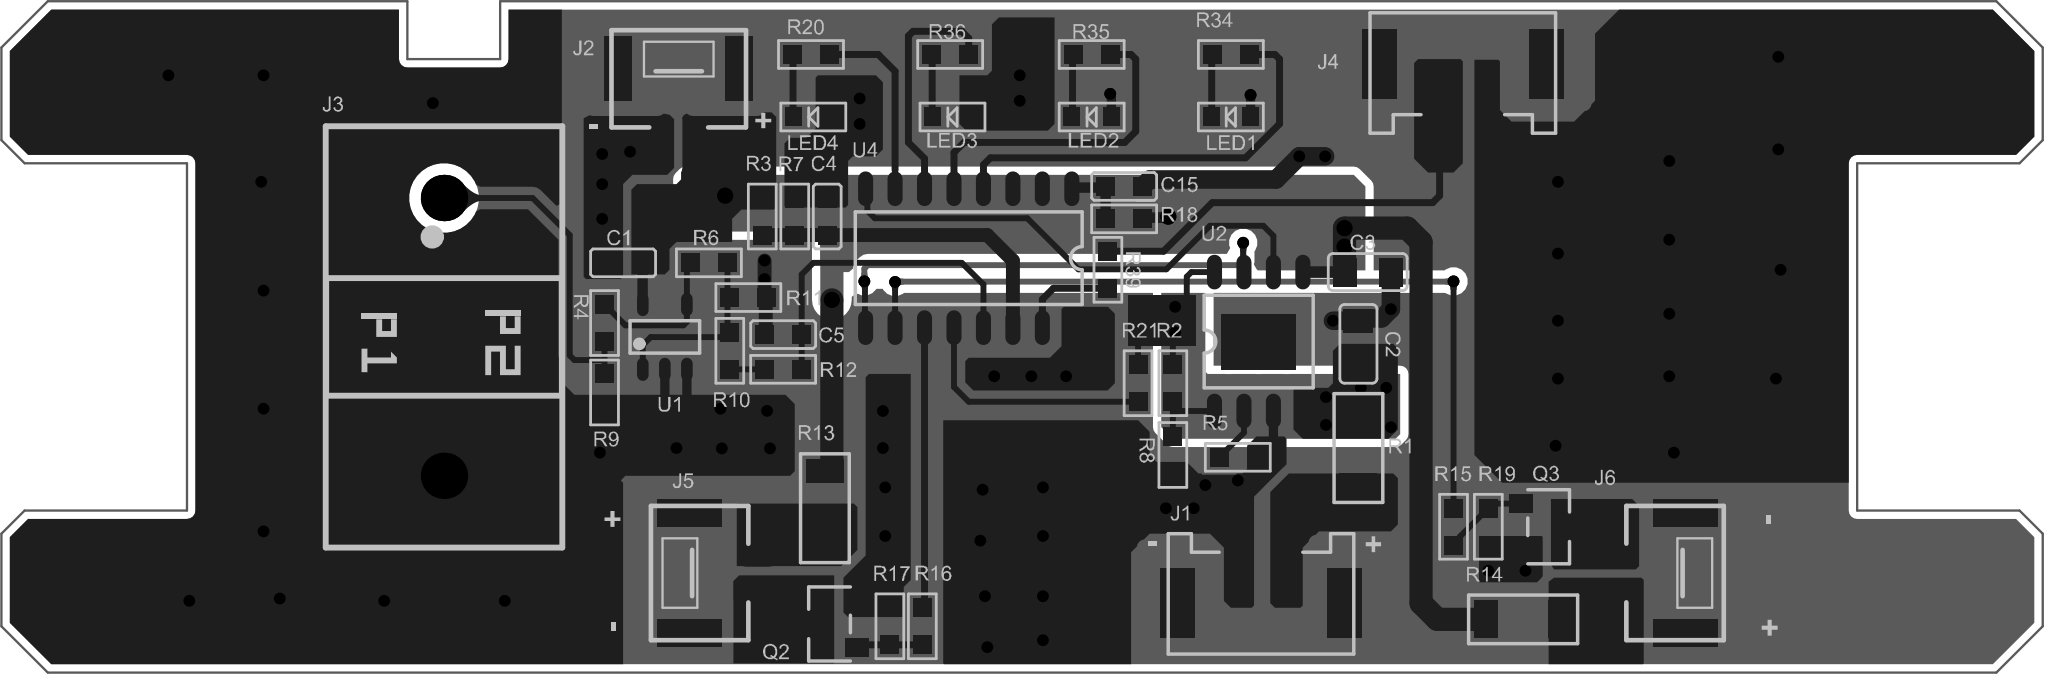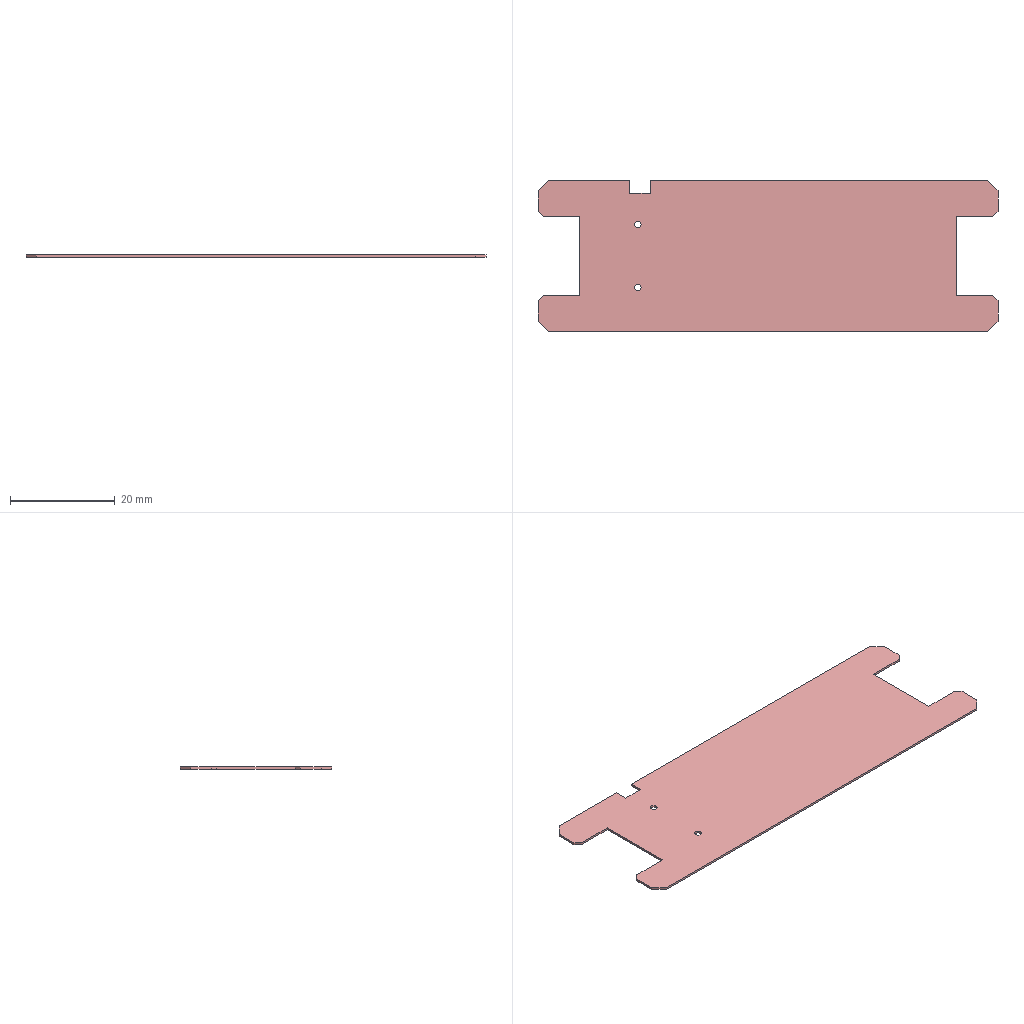Circuit board layout | Altium Designer | box 88 x 29 x 0.4 mm
Layer stack:
# Altium Designer layer stack of  (unit mm; dielectric type: 0 none, 1 core, 2 prepreg, 3 surface material)
index,name,kind,layer,copper_thickness_mm,dielectric_type,dielectric_thickness_mm,dielectric_material,dielectric_constant
0,Top Paste,other,,,,,,
1,Top Overlay,other,,,,,,
2,Top Solder,dielectric,,,3,0.0102,Solder Resist,3.5
3,Top Layer,copper,Top Layer,0.0356,,,,
4,Dielectric 1,dielectric,,,0,0.32,FR-4,4.8
5,Bottom Layer,copper,Bottom Layer,0.0356,,,,
6,Bottom Solder,dielectric,,,3,0.0102,Solder Resist,3.5
7,Bottom Overlay,other,,,,,,
8,Bottom Paste,other,,,,,,
# drill layer pairs: low layer,high layer
drill_pair,Top Layer,Bottom Layer
Part placement:
Designator,Comment,Layer,Footprint,Center-X(mm),Center-Y(mm),Rotation
C1,100nF/50V,TopLayer,C0603A,26.8,-9.3,0
U4,ZM072,TopLayer,SOP16L,41.7,-9.1,270
J3,Current sensor,TopLayer,IND-TH_L18.2-W10.2-P12.00-D0.9_ZHT103,19.08,-12.5,270
C15,1uF/10V,TopLayer,C0603A,48.4,-6,0
C3,10uF/10V,TopLayer,C0805A,58.9,-9.7,180
C2,10uF/10V,TopLayer,C0805A,58.5,-12.8,270
Q3,2N7002,TopLayer,SOT23-3L,66.7,-20.7,270
Q2,2N7002,TopLayer,SOT23-3L,35.7,-24.9,90
J6,Yellow LED,TopLayer,GH1.25-2PIN立贴带扣耐温260℃,71.125,-22.7,90
J5,Blue LED,TopLayer,GH1.25-2PIN立贴带扣耐温260℃,31.125,-22.7,270
J4,Test port,TopLayer,HY2.0WT-2A/P_Á¢Ìù´ø¿ÛÄÍÎÂ260¡æ,63,-1.9,180
J2,Battery,TopLayer,GH1.25-2PIN立贴带扣耐温260℃,29.2,-2.375,180
J1,Charge,TopLayer,HY2.0WT-2A/P_Á¢Ìù´ø¿ÛÄÍÎÂ260¡æ,54.3,-22.8,0
LED4,100%,TopLayer,LED0603A,35,-3,0
LED3,75%,TopLayer,LED0603A,41,-3,0
LED2,50%,TopLayer,LED0603A,47,-3,0
LED1,25%,TopLayer,LED0603A,53,-3,0
U2,4056,TopLayer,ESOP-8L,54.2,-12.7,90
U1,LM321,TopLayer,SOT23-5A,28.6,-12.5,90
R14,10R/1206,TopLayer,R1206A,65.6,-24.7,0
R13,10R/1206,TopLayer,R1206A,35.5,-19.9,270
R12,0R/0603,TopLayer,R0603A,33.7,-13.9,0
R11,10K/0603,TopLayer,R0603A,32.2,-10.8,0
R10,1K/0603,TopLayer,R0603A,31.4,-13.1,270
R9,2K/0603,TopLayer,R0603A,26,-14.9,270
R8,NC,TopLayer,R0603A,50.5,-17.6,90
R7,200K/0603 1%,TopLayer,R0603A,34.2,-7.3,270
R6,150K/0603,TopLayer,R0603A,30.5,-9.3,0
R5,1.2K/0603,TopLayer,R0603A,53.3,-17.7,180
R4,1K/0603,TopLayer,R0603A,26,-11.9,270
R3,510K/0603 1%,TopLayer,R0603A,32.8,-7.3,90
R2,NC,TopLayer,R0603A,50.5,-14.5,90
R1,0.5R/1206,TopLayer,R1206A,58.5,-17.3,90
C5,NC,TopLayer,C0603A,33.7,-12.4,0
C4,100nF/50V,TopLayer,C0603A,35.6,-7.3,270
R39,1K,TopLayer,R0603A,47.7,-9.6,90
R36,100R/5%,TopLayer,R0603A,40.9,-0.3,0
R35,100R/5%,TopLayer,R0603A,47,-0.3,0
R34,100R/5%,TopLayer,R0603A,53,-0.3,0
R21,NC,TopLayer,R0603A,49,-14.5,90
R20,100R/5%,TopLayer,R0603A,34.9,-0.3,0
R19,100K,TopLayer,R0603A,64.1,-20.7,90
R18,1R,TopLayer,R0603A,48.4,-7.4,180
R17,100K,TopLayer,R0603A,38.3,-25,270
R16,1K,TopLayer,R0603A,39.7,-25,90
R15,1K,TopLayer,R0603A,62.6,-20.7,90
Pad and via stacks:
# Altium Designer via and pad stacks of  (unit mm). Each distinct definition once, with the count of objects using it.
# via: kind,start_layer,end_layer,hole_mm,diameter_mm,mode(0 simple;1 top-mid-bottom;2 full stack),diameter_per_layer,count,example_net
# pad: kind,layer,hole_mm,hole_type(0 round;1 square;2 slot),plating,top_size,top_shape(1 round;2 rect;3 octagon;9 rounded rect),mid_size,bottom_size,mode,footprint,size_per_layer,count,example
pad,Top Layer,0,0,plated,1x1,1,1x1,1x1,0,,,2,3
pad,Top Layer,0,0,plated,3x1.5,2,3x1.5,3x1.5,0,HY2.0WT-2A/P \u00C1\u00A2\u00CC\u00F9\u00B4\u00F8\u00BF\u00DB\u00C4\u00CD\u00CE\u00C2260\u00A1\u00E6,,4,J4.0
pad,Top Layer,0,0,plated,4.5x0.8,1,4.5x0.8,4.5x0.8,0,HY2.0WT-2A/P \u00C1\u00A2\u00CC\u00F9\u00B4\u00F8\u00BF\u00DB\u00C4\u00CD\u00CE\u00C2260\u00A1\u00E6,,4,J4.1
pad,Top Layer,0,0,plated,0.7x0.8,2,0.7x0.8,0.7x0.8,0,LED0603A,,8,LED1.2
pad,Top Layer,0,0,plated,0.8x0.8,2,0.8x0.8,0.8x0.8,0,R0603A,,44,R17.1
pad,Top Layer,0,0,plated,0.8x1,2,0.8x1,0.8x1,0,SOT23-3L,,6,Q2.1
pad,Top Layer,0,0,plated,1x1.25,2,1x1.25,1x1.25,0,C0805A,,4,C3.2
pad,Top Layer,0,0,plated,1x1.6,2,1x1.6,1x1.6,0,R1206A,,6,R1.1
pad,Top Layer,0,0,plated,0.8x0.8,2,0.8x0.8,0.8x0.8,0,C0603A,,8,C15.2
pad,Top Layer,0,0,plated,1.7x0.7,1,1.7x0.7,1.7x0.7,0,GH1.25-2PIN\u00C1\u00A2\u00CC\u00F9\u00B4\u00F8\u00BF\u00DB\u00C4\u00CD\u00CE\u00C2260\u00A1\u00E6,,6,J5.1
pad,Top Layer,0,0,plated,2.8x1.2,2,2.8x1.2,2.8x1.2,0,GH1.25-2PIN\u00C1\u00A2\u00CC\u00F9\u00B4\u00F8\u00BF\u00DB\u00C4\u00CD\u00CE\u00C2260\u00A1\u00E6,,6,J5.0
pad,Top Layer,0,0,plated,1x0.5,1,1x0.5,1x0.5,0,SOT23-5A,,5,U1.4
pad,Top Layer,0,2,plated,0.65x1.5,1,0.65x1.5,0.65x1.5,0,SOP16L,,16,U4.12
pad,Top Layer,0,2,plated,2.4x3.2,2,2.4x3.2,2.4x3.2,0,ESOP-8L,,1,U2.0
pad,Top Layer,0,2,plated,0.65x1.5,1,0.65x1.5,0.65x1.5,0,ESOP-8L,,8,U2.1
pad,Multi-Layer,1.3,0,plated,2x2,1,2x2,2x2,0,IND-TH_L18.2-W10.2-P12.00-D0.9_ZHT103,,2,J3.1
via,Top Layer,Bottom Layer,0.3048,0.508,0,,88,GND
via,Top Layer,Bottom Layer,0.5,0.7,0,,5,BAT+
Copper pours:
name,layer,net,type(0 solid;1 hatched;2 none)
NONET_L02_P-001,Top Layer,GND,0
NONET_L02_P-001,Top Layer,GND,0
NONET_L02_P-001,Top Layer,NetJ1_2,0
NONET_L02_P-001,Top Layer,GND,0
NONET_L02_P-001,Top Layer,NetJ4_2,0
NONET_L02_P-001,Top Layer,GND,0
NONET_L02_P-001,Top Layer,GND,0
NONET_L02_P-001,Top Layer,GND,0
NONET_L02_P-001,Top Layer,EN,0
NONET_L02_P-001,Top Layer,EN,0
NONET_L02_P-001,Top Layer,NetJ6_2,0
NONET_L02_P-001,Top Layer,NetJ6_1,0
NONET_L02_P-001,Top Layer,GND,0
NONET_L02_P-001,Top Layer,GND,0
NONET_L02_P-001,Top Layer,NetJ5_1,0
NONET_L02_P-001,Top Layer,NetJ5_2,0
NONET_L02_P-001,Top Layer,BAT+,0
NONET_L02_P-001,Top Layer,GND,0
GND_L02_P015,Bottom Layer,GND,0
NONET_L02_P-001,Bottom Layer,EN,0
NONET_L02_P-001,Bottom Layer,BAT+,0
Design rules, without the lines most boards share:
# Altium Designer design rules of  (exported by Altium Designer, unit mm)
# columns: name | kind | enabled | priority | scope1 | scope2 | descriptor | typed fields (field=value)
Schematic Supply Nets | 41 | enabled | 1 | InNet('GND') | All | Supply Net(s)(InNet('GND')) |
NetAntennae | 56 | enabled | 1 | All | All | Net Antennae (Tolerance=0mm) (All) |
SilkToSilkClearance | 55 | enabled | 1 | All | All | Silk to Silk (Clearance=0mm) (All),(All) |
SilkToSolderMaskClearance | 54 | enabled | 1 | IsPad | All | Silk To Solder Mask (Clearance=0mm) (IsPad),(All) |
MinimumSolderMaskSliver | 53 | enabled | 1 | All | All | Minimum Solder Mask Sliver (Gap=0.254mm) (All),(All) |
HoleToHoleClearance | 52 | enabled | 1 | All | All | Hole To Hole Clearance (Gap=0.254mm) (All),(All) | gap=0.254
DiffPairsRouting | 51 | enabled | 1 | All | All | Differential Pairs Uncoupled Length using the Gap Constraints (Min=0.254mm) (Max=0.254mm) (Prefered=0.254mm)  and Width Constraints (Min=0.381mm) (Max=0.381mm) (Prefered=0.381mm) (All) |
HoleSize | 42 | enabled | 1 | All | All | Hole Size Constraint (Min=0.025mm) (Max=2.54mm) (All) |
Height | 50 | enabled | 1 | All | All | Height Constraint (Min=0mm) (Max=25.4mm) (Prefered=12.7mm) (All) | min_height=0 max_height=25.4
ComponentClearance | 24 | enabled | 1 | All | All | Component Clearance Constraint ( Horizontal Gap = 0.254mm, Vertical Gap = 0.254mm ) (All),(All)  | gap=0.254
SolderMaskExpansion | 13 | enabled | 1 | All | All | Solder Mask Expansion (Expansion =0.102mm) (All) | expansion=0.1016
PasteMaskExpansion | 14 | enabled | 1 | All | All | Paste Mask Expansion (Expansion =0mm) (All) | expansion=0
RoutingVias | 11 | enabled | 1 | All | All | Routing Via (MinHoleWidth=0.711mm) (MaxHoleWidth=0.711mm) (PreferredHoleWidth=0.711mm) (MinWidth=1.27mm) (MaxWidth=1.27mm) (PreferedWidth=1.27mm) (All) | via_min_hole=0.7112 via_max_hole=0.7112 via_preferred_diameter=1.27 via_preferred_hole=0.7112
RoutingCorners | 10 | enabled | 1 | All | All | Routing Corners (Style=45-Degree) (Min Setback=2.54mm) (Max Setback=2.54mm) (All) |
Width | 2 | enabled | 1 | All | All | Width Constraint (Min=0.254mm) (Max=1mm) (Preferred=0.254mm) (All) |
PolygonConnect | 20 | enabled | 1 | All | All | Polygon Connect Rule(Direct Connect )(Conductor Width=0.254mm) (Relief Angle=90 Angle) (Entries=4) (Air Gap Width=0.254mm) (All),(All) | connect_style(0=relief,1=direct,2=none)=1 relief_conductor_width=0.254 relief_entries=4
PlaneClearance | 12 | enabled | 1 | All | All | Power Plane Clearance (Clearance =0.508mm) (All) | clearance=0.508
PlaneConnect | 6 | enabled | 1 | All | All | Power Plane Connect Rule(Relief Connect )(Expansion=0.508mm) (Conductor Width=0.254mm) (Air Gap=0.254mm) (Entries=4) (All) | relief_conductor_width=0.254 relief_entries=4 relief_expansion=0.508
Clearance | 0 | enabled | 1 | All | All | Clearance Constraint (Gap=0.254mm) (All),(All) | gap=0.254
Classes set for this board:
# Altium Designer classes of  (member kind: 0 net, 1 component, 2 from-to, 3 pad, 4 layer, 5 differential pair, 6 design channel, 7 polygon, 8 structure, 9 xSignal)
# columns: class name | member kind | superclass | members
XW05 V0(YK) | 1 | no | C1; C2; C3; C4; C5; J1; J2; J3; J4; J5; J6; LED1; LED2; LED3; LED4; Q2; Q3; R1; R2; R3; R4; R5; R6; R7; R8; R9; R10; R11; R12; R13; R14; R15; R16; R17; R18; R19; R20; R21; R34; R35; R36; R39; U1; U2; U4; C4; C5; R1; R2; R3; R4; R5; R6; R7; R8; R9; R10; R11; R12; R13; R14; U1; U2; LED1; LED2; LED3; LED4; J1; J2; J4; J5; J6; Q2; Q3; C2; C3; J3; U4; C1; C15;